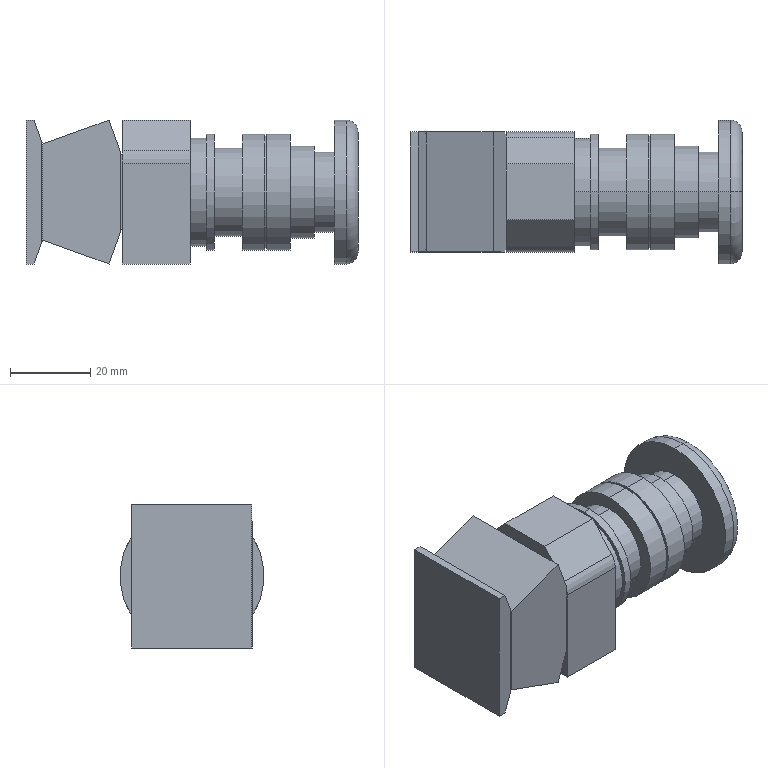Part | STEP file | Yijia emergency stop switch | 1 solid | 62 faces | box 83 x 36 x 36 mm | volume 62929 mm3 | plane 40 | cylinder 20 | torus 2 | commonest cylinder face diameters 29 x6 10 x2 20 x2 22 x2 23 x2 27 x2